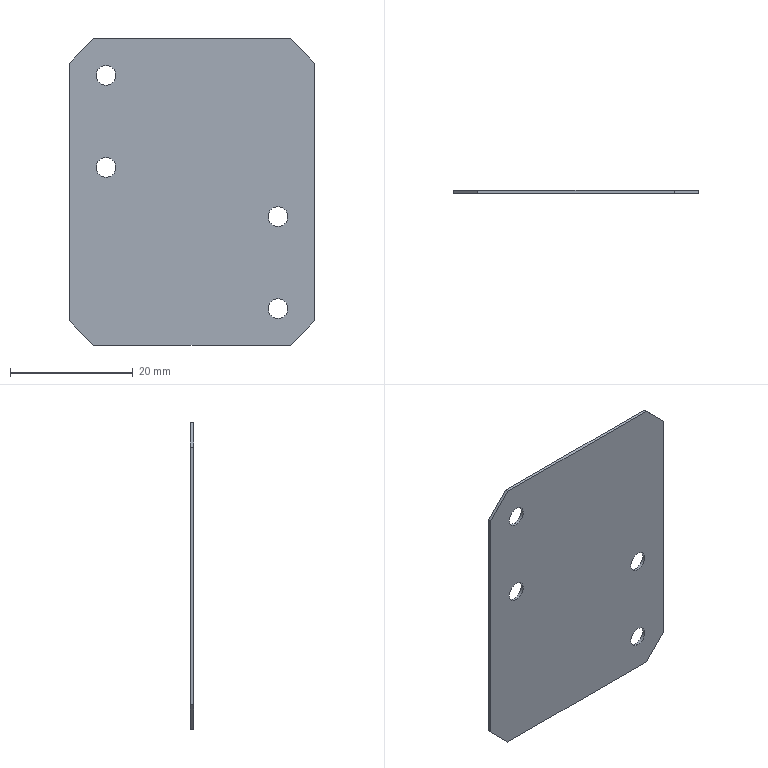Part | SolidWorks | features BaseBody 1 | 1 solid | 18 faces | box 40 x 0.5 x 50 mm | volume 967.915 mm3 | plane 10 | cylinder 8 | commonest cylinder face diameters 3.2 x8
STEP:
#1=CARTESIAN_POINT('',(14.,0.5,-20.6));
#2=VERTEX_POINT('',#1);
#3=CARTESIAN_POINT('',(14.,0.5,-17.4));
#4=VERTEX_POINT('',#3);
#5=CARTESIAN_POINT('',(14.,0.5,-19.));
#6=DIRECTION('',(0.,1.,0.));
#7=DIRECTION('',(0.,0.,-1.));
#8=AXIS2_PLACEMENT_3D('',#5,#6,#7);
#9=CIRCLE('',#8,1.6);
#10=EDGE_CURVE('',#2,#4,#9,.T.);
#11=ORIENTED_EDGE('',*,*,#10,.T.);
#12=CARTESIAN_POINT('',(14.,0.,-17.4));
#13=VERTEX_POINT('',#12);
#14=CARTESIAN_POINT('',(14.,0.5,-17.4));
#15=DIRECTION('',(0.,-1.,0.));
#16=VECTOR('',#15,1000.);
#17=LINE('',#14,#16);
#18=EDGE_CURVE('',#4,#13,#17,.T.);
#19=ORIENTED_EDGE('',*,*,#18,.T.);
#20=CARTESIAN_POINT('',(14.,0.,-20.6));
#21=VERTEX_POINT('',#20);
#22=CARTESIAN_POINT('',(14.,0.,-19.));
#23=DIRECTION('',(0.,-1.,0.));
#24=DIRECTION('',(0.,0.,-1.));
#25=AXIS2_PLACEMENT_3D('',#22,#23,#24);
#26=CIRCLE('',#25,1.6);
#27=EDGE_CURVE('',#13,#21,#26,.T.);
#28=ORIENTED_EDGE('',*,*,#27,.T.);
#29=CARTESIAN_POINT('',(14.,0.5,-20.6));
#30=DIRECTION('',(0.,-1.,0.));
#31=VECTOR('',#30,1000.);
#32=LINE('',#29,#31);
#33=EDGE_CURVE('',#2,#21,#32,.T.);
#34=ORIENTED_EDGE('',*,*,#33,.F.);
#35=EDGE_LOOP('',(#11,#19,#28,#34));
#36=FACE_OUTER_BOUND('',#35,.T.);
#37=CARTESIAN_POINT('',(14.,0.5,-19.));
#38=DIRECTION('',(0.,-1.,0.));
#39=DIRECTION('',(0.,0.,-1.));
#40=AXIS2_PLACEMENT_3D('',#37,#38,#39);
#41=CYLINDRICAL_SURFACE('',#40,1.6);
#42=ADVANCED_FACE('',(#36),#41,.F.);
#43=CARTESIAN_POINT('',(-14.,0.5,5.6));
#44=VERTEX_POINT('',#43);
#45=CARTESIAN_POINT('',(-14.,0.5,2.4));
#46=VERTEX_POINT('',#45);
#47=CARTESIAN_POINT('',(-14.,0.5,4.));
#48=DIRECTION('',(0.,-1.,0.));
#49=DIRECTION('',(0.,0.,-1.));
#50=AXIS2_PLACEMENT_3D('',#47,#48,#49);
#51=CIRCLE('',#50,1.6);
#52=EDGE_CURVE('',#44,#46,#51,.T.);
#53=ORIENTED_EDGE('',*,*,#52,.F.);
#54=CARTESIAN_POINT('',(-14.,0.,5.6));
#55=VERTEX_POINT('',#54);
#56=CARTESIAN_POINT('',(-14.,0.5,5.6));
#57=DIRECTION('',(0.,-1.,0.));
#58=VECTOR('',#57,1000.);
#59=LINE('',#56,#58);
#60=EDGE_CURVE('',#44,#55,#59,.T.);
#61=ORIENTED_EDGE('',*,*,#60,.T.);
#62=CARTESIAN_POINT('',(-14.,0.,2.4));
#63=VERTEX_POINT('',#62);
#64=CARTESIAN_POINT('',(-14.,0.,4.));
#65=DIRECTION('',(0.,-1.,0.));
#66=DIRECTION('',(0.,0.,-1.));
#67=AXIS2_PLACEMENT_3D('',#64,#65,#66);
#68=CIRCLE('',#67,1.6);
#69=EDGE_CURVE('',#55,#63,#68,.T.);
#70=ORIENTED_EDGE('',*,*,#69,.T.);
#71=CARTESIAN_POINT('',(-14.,0.5,2.4));
#72=DIRECTION('',(0.,-1.,0.));
#73=VECTOR('',#72,1000.);
#74=LINE('',#71,#73);
#75=EDGE_CURVE('',#46,#63,#74,.T.);
#76=ORIENTED_EDGE('',*,*,#75,.F.);
#77=EDGE_LOOP('',(#53,#61,#70,#76));
#78=FACE_OUTER_BOUND('',#77,.T.);
#79=CARTESIAN_POINT('',(-14.,0.5,4.));
#80=DIRECTION('',(0.,-1.,0.));
#81=DIRECTION('',(0.,0.,-1.));
#82=AXIS2_PLACEMENT_3D('',#79,#80,#81);
#83=CYLINDRICAL_SURFACE('',#82,1.6);
#84=ADVANCED_FACE('',(#78),#83,.F.);
#85=CARTESIAN_POINT('',(-14.,0.5,20.6));
#86=VERTEX_POINT('',#85);
#87=CARTESIAN_POINT('',(-14.,0.5,17.4));
#88=VERTEX_POINT('',#87);
#89=CARTESIAN_POINT('',(-14.,0.5,19.));
#90=DIRECTION('',(0.,-1.,0.));
#91=DIRECTION('',(0.,0.,-1.));
#92=AXIS2_PLACEMENT_3D('',#89,#90,#91);
#93=CIRCLE('',#92,1.6);
#94=EDGE_CURVE('',#86,#88,#93,.T.);
#95=ORIENTED_EDGE('',*,*,#94,.F.);
#96=CARTESIAN_POINT('',(-14.,0.,20.6));
#97=VERTEX_POINT('',#96);
#98=CARTESIAN_POINT('',(-14.,0.5,20.6));
#99=DIRECTION('',(0.,-1.,0.));
#100=VECTOR('',#99,1000.);
#101=LINE('',#98,#100);
#102=EDGE_CURVE('',#86,#97,#101,.T.);
#103=ORIENTED_EDGE('',*,*,#102,.T.);
#104=CARTESIAN_POINT('',(-14.,0.,17.4));
#105=VERTEX_POINT('',#104);
#106=CARTESIAN_POINT('',(-14.,0.,19.));
#107=DIRECTION('',(0.,-1.,0.));
#108=DIRECTION('',(0.,0.,-1.));
#109=AXIS2_PLACEMENT_3D('',#106,#107,#108);
#110=CIRCLE('',#109,1.6);
#111=EDGE_CURVE('',#97,#105,#110,.T.);
#112=ORIENTED_EDGE('',*,*,#111,.T.);
#113=CARTESIAN_POINT('',(-14.,0.5,17.4));
#114=DIRECTION('',(0.,-1.,0.));
#115=VECTOR('',#114,1000.);
#116=LINE('',#113,#115);
#117=EDGE_CURVE('',#88,#105,#116,.T.);
#118=ORIENTED_EDGE('',*,*,#117,.F.);
#119=EDGE_LOOP('',(#95,#103,#112,#118));
#120=FACE_OUTER_BOUND('',#119,.T.);
#121=CARTESIAN_POINT('',(-14.,0.5,19.));
#122=DIRECTION('',(0.,-1.,0.));
#123=DIRECTION('',(0.,0.,-1.));
#124=AXIS2_PLACEMENT_3D('',#121,#122,#123);
#125=CYLINDRICAL_SURFACE('',#124,1.6);
#126=ADVANCED_FACE('',(#120),#125,.F.);
#127=CARTESIAN_POINT('',(14.,0.5,-2.4));
#128=VERTEX_POINT('',#127);
#129=CARTESIAN_POINT('',(14.,0.5,-5.6));
#130=VERTEX_POINT('',#129);
#131=CARTESIAN_POINT('',(14.,0.5,-4.));
#132=DIRECTION('',(0.,-1.,0.));
#133=DIRECTION('',(0.,0.,-1.));
#134=AXIS2_PLACEMENT_3D('',#131,#132,#133);
#135=CIRCLE('',#134,1.6);
#136=EDGE_CURVE('',#128,#130,#135,.T.);
#137=ORIENTED_EDGE('',*,*,#136,.F.);
#138=CARTESIAN_POINT('',(14.,0.,-2.4));
#139=VERTEX_POINT('',#138);
#140=CARTESIAN_POINT('',(14.,0.5,-2.4));
#141=DIRECTION('',(0.,-1.,0.));
#142=VECTOR('',#141,1000.);
#143=LINE('',#140,#142);
#144=EDGE_CURVE('',#128,#139,#143,.T.);
#145=ORIENTED_EDGE('',*,*,#144,.T.);
#146=CARTESIAN_POINT('',(14.,0.,-5.6));
#147=VERTEX_POINT('',#146);
#148=CARTESIAN_POINT('',(14.,0.,-4.));
#149=DIRECTION('',(0.,-1.,0.));
#150=DIRECTION('',(0.,0.,-1.));
#151=AXIS2_PLACEMENT_3D('',#148,#149,#150);
#152=CIRCLE('',#151,1.6);
#153=EDGE_CURVE('',#139,#147,#152,.T.);
#154=ORIENTED_EDGE('',*,*,#153,.T.);
#155=CARTESIAN_POINT('',(14.,0.5,-5.6));
#156=DIRECTION('',(0.,-1.,0.));
#157=VECTOR('',#156,1000.);
#158=LINE('',#155,#157);
#159=EDGE_CURVE('',#130,#147,#158,.T.);
#160=ORIENTED_EDGE('',*,*,#159,.F.);
#161=EDGE_LOOP('',(#137,#145,#154,#160));
#162=FACE_OUTER_BOUND('',#161,.T.);
#163=CARTESIAN_POINT('',(14.,0.5,-4.));
#164=DIRECTION('',(0.,-1.,0.));
#165=DIRECTION('',(0.,0.,-1.));
#166=AXIS2_PLACEMENT_3D('',#163,#164,#165);
#167=CYLINDRICAL_SURFACE('',#166,1.6);
#168=ADVANCED_FACE('',(#162),#167,.F.);
#169=ORIENTED_EDGE('',*,*,#18,.F.);
#170=CARTESIAN_POINT('',(14.,0.5,-19.));
#171=DIRECTION('',(0.,1.,0.));
#172=DIRECTION('',(0.,0.,-1.));
#173=AXIS2_PLACEMENT_3D('',#170,#171,#172);
#174=CIRCLE('',#173,1.6);
#175=EDGE_CURVE('',#4,#2,#174,.T.);
#176=ORIENTED_EDGE('',*,*,#175,.T.);
#177=ORIENTED_EDGE('',*,*,#33,.T.);
#178=CARTESIAN_POINT('',(14.,0.,-19.));
#179=DIRECTION('',(0.,-1.,0.));
#180=DIRECTION('',(0.,0.,-1.));
#181=AXIS2_PLACEMENT_3D('',#178,#179,#180);
#182=CIRCLE('',#181,1.6);
#183=EDGE_CURVE('',#21,#13,#182,.T.);
#184=ORIENTED_EDGE('',*,*,#183,.T.);
#185=EDGE_LOOP('',(#169,#176,#177,#184));
#186=FACE_OUTER_BOUND('',#185,.T.);
#187=CARTESIAN_POINT('',(14.,0.5,-19.));
#188=DIRECTION('',(0.,-1.,0.));
#189=DIRECTION('',(0.,0.,-1.));
#190=AXIS2_PLACEMENT_3D('',#187,#188,#189);
#191=CYLINDRICAL_SURFACE('',#190,1.6);
#192=ADVANCED_FACE('',(#186),#191,.F.);
#193=ORIENTED_EDGE('',*,*,#183,.F.);
#194=ORIENTED_EDGE('',*,*,#27,.F.);
#195=EDGE_LOOP('',(#193,#194));
#196=FACE_BOUND('',#195,.T.);
#197=CARTESIAN_POINT('',(-14.,0.,4.));
#198=DIRECTION('',(0.,-1.,0.));
#199=DIRECTION('',(0.,0.,-1.));
#200=AXIS2_PLACEMENT_3D('',#197,#198,#199);
#201=CIRCLE('',#200,1.6);
#202=EDGE_CURVE('',#63,#55,#201,.T.);
#203=ORIENTED_EDGE('',*,*,#202,.F.);
#204=ORIENTED_EDGE('',*,*,#69,.F.);
#205=EDGE_LOOP('',(#203,#204));
#206=FACE_BOUND('',#205,.T.);
#207=CARTESIAN_POINT('',(-14.,0.,19.));
#208=DIRECTION('',(0.,-1.,0.));
#209=DIRECTION('',(0.,0.,-1.));
#210=AXIS2_PLACEMENT_3D('',#207,#208,#209);
#211=CIRCLE('',#210,1.6);
#212=EDGE_CURVE('',#105,#97,#211,.T.);
#213=ORIENTED_EDGE('',*,*,#212,.F.);
#214=ORIENTED_EDGE('',*,*,#111,.F.);
#215=EDGE_LOOP('',(#213,#214));
#216=FACE_BOUND('',#215,.T.);
#217=CARTESIAN_POINT('',(14.,0.,-4.));
#218=DIRECTION('',(0.,-1.,0.));
#219=DIRECTION('',(0.,0.,-1.));
#220=AXIS2_PLACEMENT_3D('',#217,#218,#219);
#221=CIRCLE('',#220,1.6);
#222=EDGE_CURVE('',#147,#139,#221,.T.);
#223=ORIENTED_EDGE('',*,*,#222,.F.);
#224=ORIENTED_EDGE('',*,*,#153,.F.);
#225=EDGE_LOOP('',(#223,#224));
#226=FACE_BOUND('',#225,.T.);
#227=CARTESIAN_POINT('',(-20.,0.,21.));
#228=VERTEX_POINT('',#227);
#229=CARTESIAN_POINT('',(-16.,0.,25.));
#230=VERTEX_POINT('',#229);
#231=CARTESIAN_POINT('',(-20.,0.,21.));
#232=DIRECTION('',(0.7071,0.,0.7071));
#233=VECTOR('',#232,1000.);
#234=LINE('',#231,#233);
#235=EDGE_CURVE('',#228,#230,#234,.T.);
#236=ORIENTED_EDGE('',*,*,#235,.F.);
#237=CARTESIAN_POINT('',(-20.,0.,-21.));
#238=VERTEX_POINT('',#237);
#239=CARTESIAN_POINT('',(-20.,0.,0.));
#240=DIRECTION('',(0.,0.,1.));
#241=VECTOR('',#240,1000.);
#242=LINE('',#239,#241);
#243=EDGE_CURVE('',#238,#228,#242,.T.);
#244=ORIENTED_EDGE('',*,*,#243,.F.);
#245=CARTESIAN_POINT('',(-16.,0.,-25.));
#246=VERTEX_POINT('',#245);
#247=CARTESIAN_POINT('',(-16.,0.,-25.));
#248=DIRECTION('',(-0.7071,0.,0.7071));
#249=VECTOR('',#248,1000.);
#250=LINE('',#247,#249);
#251=EDGE_CURVE('',#246,#238,#250,.T.);
#252=ORIENTED_EDGE('',*,*,#251,.F.);
#253=CARTESIAN_POINT('',(16.,0.,-25.));
#254=VERTEX_POINT('',#253);
#255=CARTESIAN_POINT('',(0.,0.,-25.));
#256=DIRECTION('',(-1.,0.,0.));
#257=VECTOR('',#256,1000.);
#258=LINE('',#255,#257);
#259=EDGE_CURVE('',#254,#246,#258,.T.);
#260=ORIENTED_EDGE('',*,*,#259,.F.);
#261=CARTESIAN_POINT('',(20.,0.,-21.));
#262=VERTEX_POINT('',#261);
#263=CARTESIAN_POINT('',(20.,0.,-21.));
#264=DIRECTION('',(-0.7071,0.,-0.7071));
#265=VECTOR('',#264,1000.);
#266=LINE('',#263,#265);
#267=EDGE_CURVE('',#262,#254,#266,.T.);
#268=ORIENTED_EDGE('',*,*,#267,.F.);
#269=CARTESIAN_POINT('',(20.,0.,21.));
#270=VERTEX_POINT('',#269);
#271=CARTESIAN_POINT('',(20.,0.,0.));
#272=DIRECTION('',(0.,0.,-1.));
#273=VECTOR('',#272,1000.);
#274=LINE('',#271,#273);
#275=EDGE_CURVE('',#270,#262,#274,.T.);
#276=ORIENTED_EDGE('',*,*,#275,.F.);
#277=CARTESIAN_POINT('',(16.,0.,25.));
#278=VERTEX_POINT('',#277);
#279=CARTESIAN_POINT('',(16.,0.,25.));
#280=DIRECTION('',(0.7071,0.,-0.7071));
#281=VECTOR('',#280,1000.);
#282=LINE('',#279,#281);
#283=EDGE_CURVE('',#278,#270,#282,.T.);
#284=ORIENTED_EDGE('',*,*,#283,.F.);
#285=CARTESIAN_POINT('',(0.,0.,25.));
#286=DIRECTION('',(1.,0.,0.));
#287=VECTOR('',#286,1000.);
#288=LINE('',#285,#287);
#289=EDGE_CURVE('',#230,#278,#288,.T.);
#290=ORIENTED_EDGE('',*,*,#289,.F.);
#291=EDGE_LOOP('',(#236,#244,#252,#260,#268,#276,#284,#290));
#292=FACE_OUTER_BOUND('',#291,.T.);
#293=CARTESIAN_POINT('',(20.,0.,25.));
#294=DIRECTION('',(0.,1.,0.));
#295=DIRECTION('',(0.,0.,-1.));
#296=AXIS2_PLACEMENT_3D('',#293,#294,#295);
#297=PLANE('',#296);
#298=ADVANCED_FACE('',(#196,#206,#216,#226,#292),#297,.F.);
#299=ORIENTED_EDGE('',*,*,#10,.F.);
#300=ORIENTED_EDGE('',*,*,#175,.F.);
#301=EDGE_LOOP('',(#299,#300));
#302=FACE_BOUND('',#301,.T.);
#303=CARTESIAN_POINT('',(-14.,0.5,4.));
#304=DIRECTION('',(0.,-1.,0.));
#305=DIRECTION('',(0.,0.,-1.));
#306=AXIS2_PLACEMENT_3D('',#303,#304,#305);
#307=CIRCLE('',#306,1.6);
#308=EDGE_CURVE('',#46,#44,#307,.T.);
#309=ORIENTED_EDGE('',*,*,#308,.T.);
#310=ORIENTED_EDGE('',*,*,#52,.T.);
#311=EDGE_LOOP('',(#309,#310));
#312=FACE_BOUND('',#311,.T.);
#313=CARTESIAN_POINT('',(-14.,0.5,19.));
#314=DIRECTION('',(0.,-1.,0.));
#315=DIRECTION('',(0.,0.,-1.));
#316=AXIS2_PLACEMENT_3D('',#313,#314,#315);
#317=CIRCLE('',#316,1.6);
#318=EDGE_CURVE('',#88,#86,#317,.T.);
#319=ORIENTED_EDGE('',*,*,#318,.T.);
#320=ORIENTED_EDGE('',*,*,#94,.T.);
#321=EDGE_LOOP('',(#319,#320));
#322=FACE_BOUND('',#321,.T.);
#323=CARTESIAN_POINT('',(14.,0.5,-4.));
#324=DIRECTION('',(0.,-1.,0.));
#325=DIRECTION('',(0.,0.,-1.));
#326=AXIS2_PLACEMENT_3D('',#323,#324,#325);
#327=CIRCLE('',#326,1.6);
#328=EDGE_CURVE('',#130,#128,#327,.T.);
#329=ORIENTED_EDGE('',*,*,#328,.T.);
#330=ORIENTED_EDGE('',*,*,#136,.T.);
#331=EDGE_LOOP('',(#329,#330));
#332=FACE_BOUND('',#331,.T.);
#333=CARTESIAN_POINT('',(-20.,0.5,-21.));
#334=VERTEX_POINT('',#333);
#335=CARTESIAN_POINT('',(-20.,0.5,21.));
#336=VERTEX_POINT('',#335);
#337=CARTESIAN_POINT('',(-20.,0.5,0.));
#338=DIRECTION('',(0.,0.,1.));
#339=VECTOR('',#338,1000.);
#340=LINE('',#337,#339);
#341=EDGE_CURVE('',#334,#336,#340,.T.);
#342=ORIENTED_EDGE('',*,*,#341,.T.);
#343=CARTESIAN_POINT('',(-16.,0.5,25.));
#344=VERTEX_POINT('',#343);
#345=CARTESIAN_POINT('',(-20.,0.5,21.));
#346=DIRECTION('',(0.7071,0.,0.7071));
#347=VECTOR('',#346,1000.);
#348=LINE('',#345,#347);
#349=EDGE_CURVE('',#336,#344,#348,.T.);
#350=ORIENTED_EDGE('',*,*,#349,.T.);
#351=CARTESIAN_POINT('',(16.,0.5,25.));
#352=VERTEX_POINT('',#351);
#353=CARTESIAN_POINT('',(0.,0.5,25.));
#354=DIRECTION('',(1.,0.,0.));
#355=VECTOR('',#354,1000.);
#356=LINE('',#353,#355);
#357=EDGE_CURVE('',#344,#352,#356,.T.);
#358=ORIENTED_EDGE('',*,*,#357,.T.);
#359=CARTESIAN_POINT('',(20.,0.5,21.));
#360=VERTEX_POINT('',#359);
#361=CARTESIAN_POINT('',(16.,0.5,25.));
#362=DIRECTION('',(0.7071,0.,-0.7071));
#363=VECTOR('',#362,1000.);
#364=LINE('',#361,#363);
#365=EDGE_CURVE('',#352,#360,#364,.T.);
#366=ORIENTED_EDGE('',*,*,#365,.T.);
#367=CARTESIAN_POINT('',(20.,0.5,-21.));
#368=VERTEX_POINT('',#367);
#369=CARTESIAN_POINT('',(20.,0.5,0.));
#370=DIRECTION('',(0.,0.,-1.));
#371=VECTOR('',#370,1000.);
#372=LINE('',#369,#371);
#373=EDGE_CURVE('',#360,#368,#372,.T.);
#374=ORIENTED_EDGE('',*,*,#373,.T.);
#375=CARTESIAN_POINT('',(16.,0.5,-25.));
#376=VERTEX_POINT('',#375);
#377=CARTESIAN_POINT('',(20.,0.5,-21.));
#378=DIRECTION('',(-0.7071,0.,-0.7071));
#379=VECTOR('',#378,1000.);
#380=LINE('',#377,#379);
#381=EDGE_CURVE('',#368,#376,#380,.T.);
#382=ORIENTED_EDGE('',*,*,#381,.T.);
#383=CARTESIAN_POINT('',(-16.,0.5,-25.));
#384=VERTEX_POINT('',#383);
#385=CARTESIAN_POINT('',(0.,0.5,-25.));
#386=DIRECTION('',(-1.,0.,0.));
#387=VECTOR('',#386,1000.);
#388=LINE('',#385,#387);
#389=EDGE_CURVE('',#376,#384,#388,.T.);
#390=ORIENTED_EDGE('',*,*,#389,.T.);
#391=CARTESIAN_POINT('',(-16.,0.5,-25.));
#392=DIRECTION('',(-0.7071,0.,0.7071));
#393=VECTOR('',#392,1000.);
#394=LINE('',#391,#393);
#395=EDGE_CURVE('',#384,#334,#394,.T.);
#396=ORIENTED_EDGE('',*,*,#395,.T.);
#397=EDGE_LOOP('',(#342,#350,#358,#366,#374,#382,#390,#396));
#398=FACE_OUTER_BOUND('',#397,.T.);
#399=CARTESIAN_POINT('',(20.,0.5,25.));
#400=DIRECTION('',(0.,1.,0.));
#401=DIRECTION('',(0.,0.,-1.));
#402=AXIS2_PLACEMENT_3D('',#399,#400,#401);
#403=PLANE('',#402);
#404=ADVANCED_FACE('',(#302,#312,#322,#332,#398),#403,.T.);
#405=ORIENTED_EDGE('',*,*,#60,.F.);
#406=ORIENTED_EDGE('',*,*,#308,.F.);
#407=ORIENTED_EDGE('',*,*,#75,.T.);
#408=ORIENTED_EDGE('',*,*,#202,.T.);
#409=EDGE_LOOP('',(#405,#406,#407,#408));
#410=FACE_OUTER_BOUND('',#409,.T.);
#411=CARTESIAN_POINT('',(-14.,0.5,4.));
#412=DIRECTION('',(0.,-1.,0.));
#413=DIRECTION('',(0.,0.,-1.));
#414=AXIS2_PLACEMENT_3D('',#411,#412,#413);
#415=CYLINDRICAL_SURFACE('',#414,1.6);
#416=ADVANCED_FACE('',(#410),#415,.F.);
#417=ORIENTED_EDGE('',*,*,#102,.F.);
#418=ORIENTED_EDGE('',*,*,#318,.F.);
#419=ORIENTED_EDGE('',*,*,#117,.T.);
#420=ORIENTED_EDGE('',*,*,#212,.T.);
#421=EDGE_LOOP('',(#417,#418,#419,#420));
#422=FACE_OUTER_BOUND('',#421,.T.);
#423=CARTESIAN_POINT('',(-14.,0.5,19.));
#424=DIRECTION('',(0.,-1.,0.));
#425=DIRECTION('',(0.,0.,-1.));
#426=AXIS2_PLACEMENT_3D('',#423,#424,#425);
#427=CYLINDRICAL_SURFACE('',#426,1.6);
#428=ADVANCED_FACE('',(#422),#427,.F.);
#429=ORIENTED_EDGE('',*,*,#144,.F.);
#430=ORIENTED_EDGE('',*,*,#328,.F.);
#431=ORIENTED_EDGE('',*,*,#159,.T.);
#432=ORIENTED_EDGE('',*,*,#222,.T.);
#433=EDGE_LOOP('',(#429,#430,#431,#432));
#434=FACE_OUTER_BOUND('',#433,.T.);
#435=CARTESIAN_POINT('',(14.,0.5,-4.));
#436=DIRECTION('',(0.,-1.,0.));
#437=DIRECTION('',(0.,0.,-1.));
#438=AXIS2_PLACEMENT_3D('',#435,#436,#437);
#439=CYLINDRICAL_SURFACE('',#438,1.6);
#440=ADVANCED_FACE('',(#434),#439,.F.);
#441=CARTESIAN_POINT('',(16.,0.25,25.));
#442=DIRECTION('',(0.,-1.,0.));
#443=VECTOR('',#442,1000.);
#444=LINE('',#441,#443);
#445=EDGE_CURVE('',#352,#278,#444,.T.);
#446=ORIENTED_EDGE('',*,*,#445,.F.);
#447=ORIENTED_EDGE('',*,*,#357,.F.);
#448=CARTESIAN_POINT('',(-16.,0.25,25.));
#449=DIRECTION('',(0.,1.,0.));
#450=VECTOR('',#449,1000.);
#451=LINE('',#448,#450);
#452=EDGE_CURVE('',#230,#344,#451,.T.);
#453=ORIENTED_EDGE('',*,*,#452,.F.);
#454=ORIENTED_EDGE('',*,*,#289,.T.);
#455=EDGE_LOOP('',(#446,#447,#453,#454));
#456=FACE_OUTER_BOUND('',#455,.T.);
#457=CARTESIAN_POINT('',(-16.,0.5,25.));
#458=DIRECTION('',(0.,0.,-1.));
#459=DIRECTION('',(1.,0.,0.));
#460=AXIS2_PLACEMENT_3D('',#457,#458,#459);
#461=PLANE('',#460);
#462=ADVANCED_FACE('',(#456),#461,.F.);
#463=ORIENTED_EDGE('',*,*,#452,.T.);
#464=ORIENTED_EDGE('',*,*,#349,.F.);
#465=CARTESIAN_POINT('',(-20.,0.25,21.));
#466=DIRECTION('',(0.,1.,0.));
#467=VECTOR('',#466,1000.);
#468=LINE('',#465,#467);
#469=EDGE_CURVE('',#228,#336,#468,.T.);
#470=ORIENTED_EDGE('',*,*,#469,.F.);
#471=ORIENTED_EDGE('',*,*,#235,.T.);
#472=EDGE_LOOP('',(#463,#464,#470,#471));
#473=FACE_OUTER_BOUND('',#472,.T.);
#474=CARTESIAN_POINT('',(-20.,0.5,21.));
#475=DIRECTION('',(0.7071,0.,-0.7071));
#476=DIRECTION('',(0.7071,0.,0.7071));
#477=AXIS2_PLACEMENT_3D('',#474,#475,#476);
#478=PLANE('',#477);
#479=ADVANCED_FACE('',(#473),#478,.F.);
#480=ORIENTED_EDGE('',*,*,#469,.T.);
#481=ORIENTED_EDGE('',*,*,#341,.F.);
#482=CARTESIAN_POINT('',(-20.,0.25,-21.));
#483=DIRECTION('',(0.,1.,0.));
#484=VECTOR('',#483,1000.);
#485=LINE('',#482,#484);
#486=EDGE_CURVE('',#238,#334,#485,.T.);
#487=ORIENTED_EDGE('',*,*,#486,.F.);
#488=ORIENTED_EDGE('',*,*,#243,.T.);
#489=EDGE_LOOP('',(#480,#481,#487,#488));
#490=FACE_OUTER_BOUND('',#489,.T.);
#491=CARTESIAN_POINT('',(-20.,0.5,-21.));
#492=DIRECTION('',(1.,0.,0.));
#493=DIRECTION('',(0.,0.,1.));
#494=AXIS2_PLACEMENT_3D('',#491,#492,#493);
#495=PLANE('',#494);
#496=ADVANCED_FACE('',(#490),#495,.F.);
#497=ORIENTED_EDGE('',*,*,#486,.T.);
#498=ORIENTED_EDGE('',*,*,#395,.F.);
#499=CARTESIAN_POINT('',(-16.,0.25,-25.));
#500=DIRECTION('',(0.,1.,0.));
#501=VECTOR('',#500,1000.);
#502=LINE('',#499,#501);
#503=EDGE_CURVE('',#246,#384,#502,.T.);
#504=ORIENTED_EDGE('',*,*,#503,.F.);
#505=ORIENTED_EDGE('',*,*,#251,.T.);
#506=EDGE_LOOP('',(#497,#498,#504,#505));
#507=FACE_OUTER_BOUND('',#506,.T.);
#508=CARTESIAN_POINT('',(-16.,0.5,-25.));
#509=DIRECTION('',(0.7071,0.,0.7071));
#510=DIRECTION('',(-0.7071,0.,0.7071));
#511=AXIS2_PLACEMENT_3D('',#508,#509,#510);
#512=PLANE('',#511);
#513=ADVANCED_FACE('',(#507),#512,.F.);
#514=ORIENTED_EDGE('',*,*,#503,.T.);
#515=ORIENTED_EDGE('',*,*,#389,.F.);
#516=CARTESIAN_POINT('',(16.,0.25,-25.));
#517=DIRECTION('',(0.,1.,0.));
#518=VECTOR('',#517,1000.);
#519=LINE('',#516,#518);
#520=EDGE_CURVE('',#254,#376,#519,.T.);
#521=ORIENTED_EDGE('',*,*,#520,.F.);
#522=ORIENTED_EDGE('',*,*,#259,.T.);
#523=EDGE_LOOP('',(#514,#515,#521,#522));
#524=FACE_OUTER_BOUND('',#523,.T.);
#525=CARTESIAN_POINT('',(16.,0.5,-25.));
#526=DIRECTION('',(0.,0.,1.));
#527=DIRECTION('',(-1.,0.,0.));
#528=AXIS2_PLACEMENT_3D('',#525,#526,#527);
#529=PLANE('',#528);
#530=ADVANCED_FACE('',(#524),#529,.F.);
#531=ORIENTED_EDGE('',*,*,#520,.T.);
#532=ORIENTED_EDGE('',*,*,#381,.F.);
#533=CARTESIAN_POINT('',(20.,0.25,-21.));
#534=DIRECTION('',(0.,1.,0.));
#535=VECTOR('',#534,1000.);
#536=LINE('',#533,#535);
#537=EDGE_CURVE('',#262,#368,#536,.T.);
#538=ORIENTED_EDGE('',*,*,#537,.F.);
#539=ORIENTED_EDGE('',*,*,#267,.T.);
#540=EDGE_LOOP('',(#531,#532,#538,#539));
#541=FACE_OUTER_BOUND('',#540,.T.);
#542=CARTESIAN_POINT('',(20.,0.5,-21.));
#543=DIRECTION('',(-0.7071,0.,0.7071));
#544=DIRECTION('',(-0.7071,0.,-0.7071));
#545=AXIS2_PLACEMENT_3D('',#542,#543,#544);
#546=PLANE('',#545);
#547=ADVANCED_FACE('',(#541),#546,.F.);
#548=ORIENTED_EDGE('',*,*,#537,.T.);
#549=ORIENTED_EDGE('',*,*,#373,.F.);
#550=CARTESIAN_POINT('',(20.,0.25,21.));
#551=DIRECTION('',(0.,1.,0.));
#552=VECTOR('',#551,1000.);
#553=LINE('',#550,#552);
#554=EDGE_CURVE('',#270,#360,#553,.T.);
#555=ORIENTED_EDGE('',*,*,#554,.F.);
#556=ORIENTED_EDGE('',*,*,#275,.T.);
#557=EDGE_LOOP('',(#548,#549,#555,#556));
#558=FACE_OUTER_BOUND('',#557,.T.);
#559=CARTESIAN_POINT('',(20.,0.5,21.));
#560=DIRECTION('',(-1.,0.,0.));
#561=DIRECTION('',(0.,0.,-1.));
#562=AXIS2_PLACEMENT_3D('',#559,#560,#561);
#563=PLANE('',#562);
#564=ADVANCED_FACE('',(#558),#563,.F.);
#565=ORIENTED_EDGE('',*,*,#554,.T.);
#566=ORIENTED_EDGE('',*,*,#365,.F.);
#567=ORIENTED_EDGE('',*,*,#445,.T.);
#568=ORIENTED_EDGE('',*,*,#283,.T.);
#569=EDGE_LOOP('',(#565,#566,#567,#568));
#570=FACE_OUTER_BOUND('',#569,.T.);
#571=CARTESIAN_POINT('',(16.,0.5,25.));
#572=DIRECTION('',(-0.7071,0.,-0.7071));
#573=DIRECTION('',(0.7071,0.,-0.7071));
#574=AXIS2_PLACEMENT_3D('',#571,#572,#573);
#575=PLANE('',#574);
#576=ADVANCED_FACE('',(#570),#575,.F.);
#577=CLOSED_SHELL('',(#42,#84,#126,#168,#192,#298,#404,#416,#428,#440,#462,#479,#496,#513,#530,#547,#564,#576));
#578=MANIFOLD_SOLID_BREP('',#577);
#579=CARTESIAN_POINT('',(0.,0.,0.));
#580=DIRECTION('',(0.,0.,1.));
#581=DIRECTION('',(1.,0.,0.));
#582=AXIS2_PLACEMENT_3D('',#579,#580,#581);
#583=(LENGTH_UNIT()NAMED_UNIT(*)SI_UNIT(.MILLI.,.METRE.));
#584=UNCERTAINTY_MEASURE_WITH_UNIT(LENGTH_MEASURE(0.00001),#583,'','');
#585=(NAMED_UNIT(*)PLANE_ANGLE_UNIT()SI_UNIT($,.RADIAN.));
#586=(NAMED_UNIT(*)SI_UNIT($,.STERADIAN.)SOLID_ANGLE_UNIT());
#587=(GEOMETRIC_REPRESENTATION_CONTEXT(3)GLOBAL_UNCERTAINTY_ASSIGNED_CONTEXT((#584))GLOBAL_UNIT_ASSIGNED_CONTEXT((#583,#585,#586))REPRESENTATION_CONTEXT('',''));
#588=ADVANCED_BREP_SHAPE_REPRESENTATION('',(#578,#582),#587);